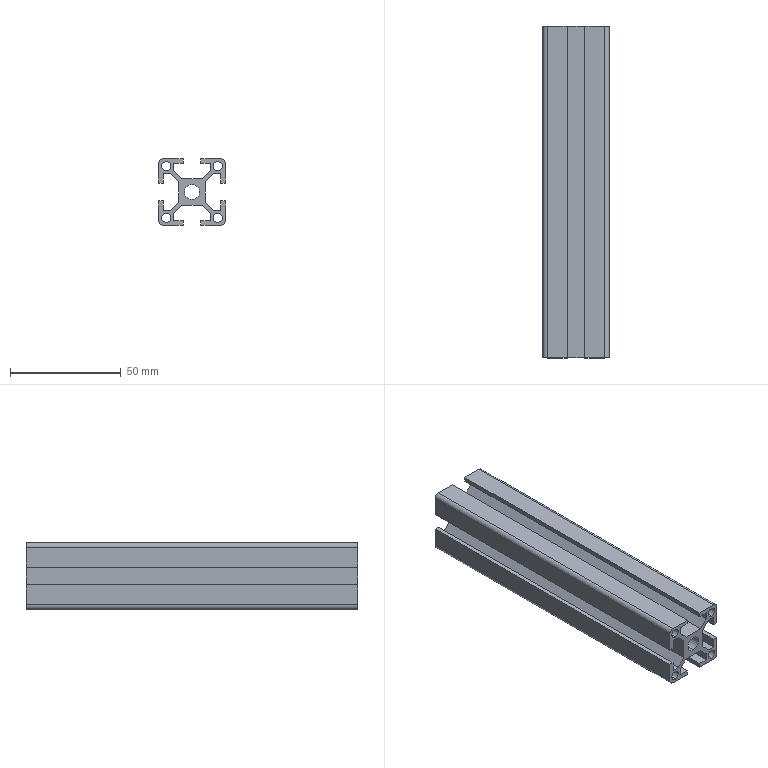Part | SolidWorks | features Extrusion 1 | 1 solid | 60 faces | box 30 x 150 x 30 mm | volume 49881 mm3 | plane 46 | cylinder 14 | commonest cylinder face diameters 4.2 x8 4 x4 6.8 x2